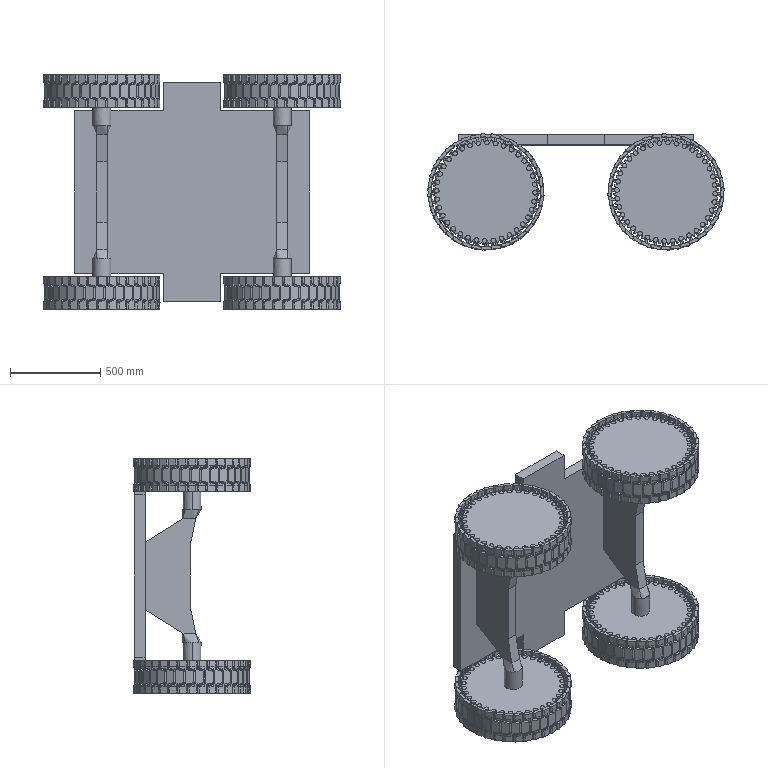Part | SolidWorks | 182 solids | 10494 faces | volume 206829671 mm3 | plane 5746 | cylinder 4684 | cone 32 | spline 16 | torus 16 | commonest cylinder face diameters 8 x1840 25 x1048 16 x864 4 x576 18 x64 20 x64